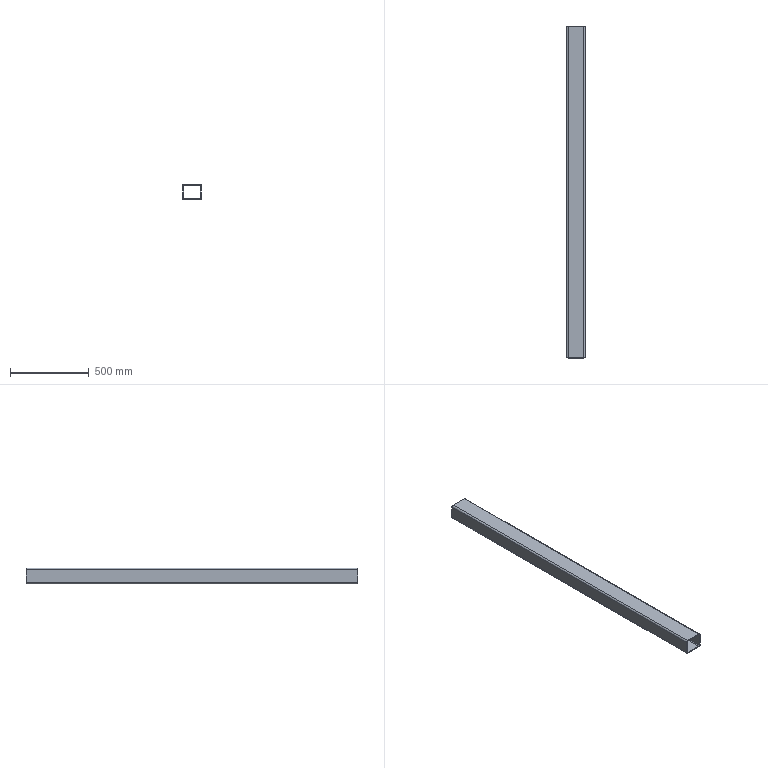Part | SolidWorks | features ExtruThin 1 | 1 solid | 18 faces | box 120 x 2114 x 100 mm | volume 5124111 mm3 | plane 10 | cylinder 8 | commonest cylinder face diameters 8 x4 20 x4
STEP:
#1=CARTESIAN_POINT('',(60.,1057.,-40.));
#2=VERTEX_POINT('',#1);
#3=CARTESIAN_POINT('',(50.,1057.,-50.));
#4=VERTEX_POINT('',#3);
#5=CARTESIAN_POINT('',(50.,1057.,-40.));
#6=DIRECTION('',(0.,1.,0.));
#7=DIRECTION('',(0.,0.,-1.));
#8=AXIS2_PLACEMENT_3D('',#5,#6,#7);
#9=CIRCLE('',#8,10.);
#10=EDGE_CURVE('',#2,#4,#9,.T.);
#11=ORIENTED_EDGE('',*,*,#10,.T.);
#12=CARTESIAN_POINT('',(-50.,1057.,-50.));
#13=VERTEX_POINT('',#12);
#14=CARTESIAN_POINT('',(-50.,1057.,-50.));
#15=DIRECTION('',(-1.,0.,0.));
#16=VECTOR('',#15,1000.);
#17=LINE('',#14,#16);
#18=EDGE_CURVE('',#4,#13,#17,.T.);
#19=ORIENTED_EDGE('',*,*,#18,.T.);
#20=CARTESIAN_POINT('',(-60.,1057.,-40.));
#21=VERTEX_POINT('',#20);
#22=CARTESIAN_POINT('',(-50.,1057.,-40.));
#23=DIRECTION('',(0.,1.,0.));
#24=DIRECTION('',(0.,0.,1.));
#25=AXIS2_PLACEMENT_3D('',#22,#23,#24);
#26=CIRCLE('',#25,10.);
#27=EDGE_CURVE('',#13,#21,#26,.T.);
#28=ORIENTED_EDGE('',*,*,#27,.T.);
#29=CARTESIAN_POINT('',(-60.,1057.,40.));
#30=VERTEX_POINT('',#29);
#31=CARTESIAN_POINT('',(-60.,1057.,-40.));
#32=DIRECTION('',(0.,0.,1.));
#33=VECTOR('',#32,1000.);
#34=LINE('',#31,#33);
#35=EDGE_CURVE('',#21,#30,#34,.T.);
#36=ORIENTED_EDGE('',*,*,#35,.T.);
#37=CARTESIAN_POINT('',(-50.,1057.,50.));
#38=VERTEX_POINT('',#37);
#39=CARTESIAN_POINT('',(-50.,1057.,40.));
#40=DIRECTION('',(0.,1.,0.));
#41=DIRECTION('',(0.,0.,1.));
#42=AXIS2_PLACEMENT_3D('',#39,#40,#41);
#43=CIRCLE('',#42,10.);
#44=EDGE_CURVE('',#30,#38,#43,.T.);
#45=ORIENTED_EDGE('',*,*,#44,.T.);
#46=CARTESIAN_POINT('',(50.,1057.,50.));
#47=VERTEX_POINT('',#46);
#48=CARTESIAN_POINT('',(-50.,1057.,50.));
#49=DIRECTION('',(1.,0.,0.));
#50=VECTOR('',#49,1000.);
#51=LINE('',#48,#50);
#52=EDGE_CURVE('',#38,#47,#51,.T.);
#53=ORIENTED_EDGE('',*,*,#52,.T.);
#54=CARTESIAN_POINT('',(60.,1057.,40.));
#55=VERTEX_POINT('',#54);
#56=CARTESIAN_POINT('',(50.,1057.,40.));
#57=DIRECTION('',(0.,1.,0.));
#58=DIRECTION('',(0.,0.,1.));
#59=AXIS2_PLACEMENT_3D('',#56,#57,#58);
#60=CIRCLE('',#59,10.);
#61=EDGE_CURVE('',#47,#55,#60,.T.);
#62=ORIENTED_EDGE('',*,*,#61,.T.);
#63=CARTESIAN_POINT('',(60.,1057.,-40.));
#64=DIRECTION('',(0.,0.,-1.));
#65=VECTOR('',#64,1000.);
#66=LINE('',#63,#65);
#67=EDGE_CURVE('',#55,#2,#66,.T.);
#68=ORIENTED_EDGE('',*,*,#67,.T.);
#69=EDGE_LOOP('',(#11,#19,#28,#36,#45,#53,#62,#68));
#70=FACE_OUTER_BOUND('',#69,.T.);
#71=CARTESIAN_POINT('',(50.,1057.,-44.));
#72=VERTEX_POINT('',#71);
#73=CARTESIAN_POINT('',(-50.,1057.,-44.));
#74=VERTEX_POINT('',#73);
#75=CARTESIAN_POINT('',(50.,1057.,-44.));
#76=DIRECTION('',(-1.,0.,0.));
#77=VECTOR('',#76,1000.);
#78=LINE('',#75,#77);
#79=EDGE_CURVE('',#72,#74,#78,.T.);
#80=ORIENTED_EDGE('',*,*,#79,.F.);
#81=CARTESIAN_POINT('',(54.,1057.,-40.));
#82=VERTEX_POINT('',#81);
#83=CARTESIAN_POINT('',(50.,1057.,-40.));
#84=DIRECTION('',(0.,1.,0.));
#85=DIRECTION('',(-1.,0.,0.));
#86=AXIS2_PLACEMENT_3D('',#83,#84,#85);
#87=CIRCLE('',#86,4.);
#88=EDGE_CURVE('',#82,#72,#87,.T.);
#89=ORIENTED_EDGE('',*,*,#88,.F.);
#90=CARTESIAN_POINT('',(54.,1057.,40.));
#91=VERTEX_POINT('',#90);
#92=CARTESIAN_POINT('',(54.,1057.,-40.));
#93=DIRECTION('',(0.,0.,-1.));
#94=VECTOR('',#93,1000.);
#95=LINE('',#92,#94);
#96=EDGE_CURVE('',#91,#82,#95,.T.);
#97=ORIENTED_EDGE('',*,*,#96,.F.);
#98=CARTESIAN_POINT('',(50.,1057.,44.));
#99=VERTEX_POINT('',#98);
#100=CARTESIAN_POINT('',(50.,1057.,40.));
#101=DIRECTION('',(0.,1.,0.));
#102=DIRECTION('',(-1.,0.,0.));
#103=AXIS2_PLACEMENT_3D('',#100,#101,#102);
#104=CIRCLE('',#103,4.);
#105=EDGE_CURVE('',#99,#91,#104,.T.);
#106=ORIENTED_EDGE('',*,*,#105,.F.);
#107=CARTESIAN_POINT('',(-50.,1057.,44.));
#108=VERTEX_POINT('',#107);
#109=CARTESIAN_POINT('',(50.,1057.,44.));
#110=DIRECTION('',(1.,0.,0.));
#111=VECTOR('',#110,1000.);
#112=LINE('',#109,#111);
#113=EDGE_CURVE('',#108,#99,#112,.T.);
#114=ORIENTED_EDGE('',*,*,#113,.F.);
#115=CARTESIAN_POINT('',(-54.,1057.,40.));
#116=VERTEX_POINT('',#115);
#117=CARTESIAN_POINT('',(-50.,1057.,40.));
#118=DIRECTION('',(0.,1.,0.));
#119=DIRECTION('',(-1.,0.,0.));
#120=AXIS2_PLACEMENT_3D('',#117,#118,#119);
#121=CIRCLE('',#120,4.);
#122=EDGE_CURVE('',#116,#108,#121,.T.);
#123=ORIENTED_EDGE('',*,*,#122,.F.);
#124=CARTESIAN_POINT('',(-54.,1057.,-40.));
#125=VERTEX_POINT('',#124);
#126=CARTESIAN_POINT('',(-54.,1057.,-40.));
#127=DIRECTION('',(0.,0.,1.));
#128=VECTOR('',#127,1000.);
#129=LINE('',#126,#128);
#130=EDGE_CURVE('',#125,#116,#129,.T.);
#131=ORIENTED_EDGE('',*,*,#130,.F.);
#132=CARTESIAN_POINT('',(-50.,1057.,-40.));
#133=DIRECTION('',(0.,1.,0.));
#134=DIRECTION('',(-1.,0.,0.));
#135=AXIS2_PLACEMENT_3D('',#132,#133,#134);
#136=CIRCLE('',#135,4.);
#137=EDGE_CURVE('',#74,#125,#136,.T.);
#138=ORIENTED_EDGE('',*,*,#137,.F.);
#139=EDGE_LOOP('',(#80,#89,#97,#106,#114,#123,#131,#138));
#140=FACE_BOUND('',#139,.T.);
#141=CARTESIAN_POINT('',(50.,1057.,-40.));
#142=DIRECTION('',(0.,1.,0.));
#143=DIRECTION('',(0.,0.,1.));
#144=AXIS2_PLACEMENT_3D('',#141,#142,#143);
#145=PLANE('',#144);
#146=ADVANCED_FACE('',(#70,#140),#145,.T.);
#147=CARTESIAN_POINT('',(60.,-1057.,-40.));
#148=VERTEX_POINT('',#147);
#149=CARTESIAN_POINT('',(50.,-1057.,-50.));
#150=VERTEX_POINT('',#149);
#151=CARTESIAN_POINT('',(50.,-1057.,-40.));
#152=DIRECTION('',(0.,1.,0.));
#153=DIRECTION('',(0.,0.,-1.));
#154=AXIS2_PLACEMENT_3D('',#151,#152,#153);
#155=CIRCLE('',#154,10.);
#156=EDGE_CURVE('',#148,#150,#155,.T.);
#157=ORIENTED_EDGE('',*,*,#156,.F.);
#158=CARTESIAN_POINT('',(60.,-1057.,40.));
#159=VERTEX_POINT('',#158);
#160=CARTESIAN_POINT('',(60.,-1057.,-40.));
#161=DIRECTION('',(0.,0.,-1.));
#162=VECTOR('',#161,1000.);
#163=LINE('',#160,#162);
#164=EDGE_CURVE('',#159,#148,#163,.T.);
#165=ORIENTED_EDGE('',*,*,#164,.F.);
#166=CARTESIAN_POINT('',(50.,-1057.,50.));
#167=VERTEX_POINT('',#166);
#168=CARTESIAN_POINT('',(50.,-1057.,40.));
#169=DIRECTION('',(0.,1.,0.));
#170=DIRECTION('',(0.,0.,1.));
#171=AXIS2_PLACEMENT_3D('',#168,#169,#170);
#172=CIRCLE('',#171,10.);
#173=EDGE_CURVE('',#167,#159,#172,.T.);
#174=ORIENTED_EDGE('',*,*,#173,.F.);
#175=CARTESIAN_POINT('',(-50.,-1057.,50.));
#176=VERTEX_POINT('',#175);
#177=CARTESIAN_POINT('',(-50.,-1057.,50.));
#178=DIRECTION('',(1.,0.,0.));
#179=VECTOR('',#178,1000.);
#180=LINE('',#177,#179);
#181=EDGE_CURVE('',#176,#167,#180,.T.);
#182=ORIENTED_EDGE('',*,*,#181,.F.);
#183=CARTESIAN_POINT('',(-60.,-1057.,40.));
#184=VERTEX_POINT('',#183);
#185=CARTESIAN_POINT('',(-50.,-1057.,40.));
#186=DIRECTION('',(0.,1.,0.));
#187=DIRECTION('',(0.,0.,1.));
#188=AXIS2_PLACEMENT_3D('',#185,#186,#187);
#189=CIRCLE('',#188,10.);
#190=EDGE_CURVE('',#184,#176,#189,.T.);
#191=ORIENTED_EDGE('',*,*,#190,.F.);
#192=CARTESIAN_POINT('',(-60.,-1057.,-40.));
#193=VERTEX_POINT('',#192);
#194=CARTESIAN_POINT('',(-60.,-1057.,-40.));
#195=DIRECTION('',(0.,0.,1.));
#196=VECTOR('',#195,1000.);
#197=LINE('',#194,#196);
#198=EDGE_CURVE('',#193,#184,#197,.T.);
#199=ORIENTED_EDGE('',*,*,#198,.F.);
#200=CARTESIAN_POINT('',(-50.,-1057.,-50.));
#201=VERTEX_POINT('',#200);
#202=CARTESIAN_POINT('',(-50.,-1057.,-40.));
#203=DIRECTION('',(0.,1.,0.));
#204=DIRECTION('',(0.,0.,1.));
#205=AXIS2_PLACEMENT_3D('',#202,#203,#204);
#206=CIRCLE('',#205,10.);
#207=EDGE_CURVE('',#201,#193,#206,.T.);
#208=ORIENTED_EDGE('',*,*,#207,.F.);
#209=CARTESIAN_POINT('',(-50.,-1057.,-50.));
#210=DIRECTION('',(-1.,0.,0.));
#211=VECTOR('',#210,1000.);
#212=LINE('',#209,#211);
#213=EDGE_CURVE('',#150,#201,#212,.T.);
#214=ORIENTED_EDGE('',*,*,#213,.F.);
#215=EDGE_LOOP('',(#157,#165,#174,#182,#191,#199,#208,#214));
#216=FACE_OUTER_BOUND('',#215,.T.);
#217=CARTESIAN_POINT('',(54.,-1057.,-40.));
#218=VERTEX_POINT('',#217);
#219=CARTESIAN_POINT('',(50.,-1057.,-44.));
#220=VERTEX_POINT('',#219);
#221=CARTESIAN_POINT('',(50.,-1057.,-40.));
#222=DIRECTION('',(0.,1.,0.));
#223=DIRECTION('',(-1.,0.,0.));
#224=AXIS2_PLACEMENT_3D('',#221,#222,#223);
#225=CIRCLE('',#224,4.);
#226=EDGE_CURVE('',#218,#220,#225,.T.);
#227=ORIENTED_EDGE('',*,*,#226,.T.);
#228=CARTESIAN_POINT('',(-50.,-1057.,-44.));
#229=VERTEX_POINT('',#228);
#230=CARTESIAN_POINT('',(50.,-1057.,-44.));
#231=DIRECTION('',(-1.,0.,0.));
#232=VECTOR('',#231,1000.);
#233=LINE('',#230,#232);
#234=EDGE_CURVE('',#220,#229,#233,.T.);
#235=ORIENTED_EDGE('',*,*,#234,.T.);
#236=CARTESIAN_POINT('',(-54.,-1057.,-40.));
#237=VERTEX_POINT('',#236);
#238=CARTESIAN_POINT('',(-50.,-1057.,-40.));
#239=DIRECTION('',(0.,1.,0.));
#240=DIRECTION('',(-1.,0.,0.));
#241=AXIS2_PLACEMENT_3D('',#238,#239,#240);
#242=CIRCLE('',#241,4.);
#243=EDGE_CURVE('',#229,#237,#242,.T.);
#244=ORIENTED_EDGE('',*,*,#243,.T.);
#245=CARTESIAN_POINT('',(-54.,-1057.,40.));
#246=VERTEX_POINT('',#245);
#247=CARTESIAN_POINT('',(-54.,-1057.,-40.));
#248=DIRECTION('',(0.,0.,1.));
#249=VECTOR('',#248,1000.);
#250=LINE('',#247,#249);
#251=EDGE_CURVE('',#237,#246,#250,.T.);
#252=ORIENTED_EDGE('',*,*,#251,.T.);
#253=CARTESIAN_POINT('',(-50.,-1057.,44.));
#254=VERTEX_POINT('',#253);
#255=CARTESIAN_POINT('',(-50.,-1057.,40.));
#256=DIRECTION('',(0.,1.,0.));
#257=DIRECTION('',(-1.,0.,0.));
#258=AXIS2_PLACEMENT_3D('',#255,#256,#257);
#259=CIRCLE('',#258,4.);
#260=EDGE_CURVE('',#246,#254,#259,.T.);
#261=ORIENTED_EDGE('',*,*,#260,.T.);
#262=CARTESIAN_POINT('',(50.,-1057.,44.));
#263=VERTEX_POINT('',#262);
#264=CARTESIAN_POINT('',(50.,-1057.,44.));
#265=DIRECTION('',(1.,0.,0.));
#266=VECTOR('',#265,1000.);
#267=LINE('',#264,#266);
#268=EDGE_CURVE('',#254,#263,#267,.T.);
#269=ORIENTED_EDGE('',*,*,#268,.T.);
#270=CARTESIAN_POINT('',(54.,-1057.,40.));
#271=VERTEX_POINT('',#270);
#272=CARTESIAN_POINT('',(50.,-1057.,40.));
#273=DIRECTION('',(0.,1.,0.));
#274=DIRECTION('',(-1.,0.,0.));
#275=AXIS2_PLACEMENT_3D('',#272,#273,#274);
#276=CIRCLE('',#275,4.);
#277=EDGE_CURVE('',#263,#271,#276,.T.);
#278=ORIENTED_EDGE('',*,*,#277,.T.);
#279=CARTESIAN_POINT('',(54.,-1057.,-40.));
#280=DIRECTION('',(0.,0.,-1.));
#281=VECTOR('',#280,1000.);
#282=LINE('',#279,#281);
#283=EDGE_CURVE('',#271,#218,#282,.T.);
#284=ORIENTED_EDGE('',*,*,#283,.T.);
#285=EDGE_LOOP('',(#227,#235,#244,#252,#261,#269,#278,#284));
#286=FACE_BOUND('',#285,.T.);
#287=CARTESIAN_POINT('',(50.,-1057.,-40.));
#288=DIRECTION('',(0.,1.,0.));
#289=DIRECTION('',(0.,0.,1.));
#290=AXIS2_PLACEMENT_3D('',#287,#288,#289);
#291=PLANE('',#290);
#292=ADVANCED_FACE('',(#216,#286),#291,.F.);
#293=ORIENTED_EDGE('',*,*,#156,.T.);
#294=CARTESIAN_POINT('',(50.,1057.,-50.));
#295=DIRECTION('',(0.,-1.,0.));
#296=VECTOR('',#295,1000.);
#297=LINE('',#294,#296);
#298=EDGE_CURVE('',#4,#150,#297,.T.);
#299=ORIENTED_EDGE('',*,*,#298,.F.);
#300=ORIENTED_EDGE('',*,*,#10,.F.);
#301=CARTESIAN_POINT('',(60.,1057.,-40.));
#302=DIRECTION('',(0.,-1.,0.));
#303=VECTOR('',#302,1000.);
#304=LINE('',#301,#303);
#305=EDGE_CURVE('',#2,#148,#304,.T.);
#306=ORIENTED_EDGE('',*,*,#305,.T.);
#307=EDGE_LOOP('',(#293,#299,#300,#306));
#308=FACE_OUTER_BOUND('',#307,.T.);
#309=CARTESIAN_POINT('',(50.,1057.,-40.));
#310=DIRECTION('',(0.,-1.,0.));
#311=DIRECTION('',(0.,0.,-1.));
#312=AXIS2_PLACEMENT_3D('',#309,#310,#311);
#313=CYLINDRICAL_SURFACE('',#312,10.);
#314=ADVANCED_FACE('',(#308),#313,.T.);
#315=ORIENTED_EDGE('',*,*,#213,.T.);
#316=CARTESIAN_POINT('',(-50.,1057.,-50.));
#317=DIRECTION('',(0.,-1.,0.));
#318=VECTOR('',#317,1000.);
#319=LINE('',#316,#318);
#320=EDGE_CURVE('',#13,#201,#319,.T.);
#321=ORIENTED_EDGE('',*,*,#320,.F.);
#322=ORIENTED_EDGE('',*,*,#18,.F.);
#323=ORIENTED_EDGE('',*,*,#298,.T.);
#324=EDGE_LOOP('',(#315,#321,#322,#323));
#325=FACE_OUTER_BOUND('',#324,.T.);
#326=CARTESIAN_POINT('',(-50.,1057.,-50.));
#327=DIRECTION('',(0.,0.,1.));
#328=DIRECTION('',(1.,0.,0.));
#329=AXIS2_PLACEMENT_3D('',#326,#327,#328);
#330=PLANE('',#329);
#331=ADVANCED_FACE('',(#325),#330,.F.);
#332=ORIENTED_EDGE('',*,*,#207,.T.);
#333=CARTESIAN_POINT('',(-60.,1057.,-40.));
#334=DIRECTION('',(0.,-1.,0.));
#335=VECTOR('',#334,1000.);
#336=LINE('',#333,#335);
#337=EDGE_CURVE('',#21,#193,#336,.T.);
#338=ORIENTED_EDGE('',*,*,#337,.F.);
#339=ORIENTED_EDGE('',*,*,#27,.F.);
#340=ORIENTED_EDGE('',*,*,#320,.T.);
#341=EDGE_LOOP('',(#332,#338,#339,#340));
#342=FACE_OUTER_BOUND('',#341,.T.);
#343=CARTESIAN_POINT('',(-50.,1057.,-40.));
#344=DIRECTION('',(0.,-1.,0.));
#345=DIRECTION('',(0.,0.,-1.));
#346=AXIS2_PLACEMENT_3D('',#343,#344,#345);
#347=CYLINDRICAL_SURFACE('',#346,10.);
#348=ADVANCED_FACE('',(#342),#347,.T.);
#349=ORIENTED_EDGE('',*,*,#198,.T.);
#350=CARTESIAN_POINT('',(-60.,1057.,40.));
#351=DIRECTION('',(0.,-1.,0.));
#352=VECTOR('',#351,1000.);
#353=LINE('',#350,#352);
#354=EDGE_CURVE('',#30,#184,#353,.T.);
#355=ORIENTED_EDGE('',*,*,#354,.F.);
#356=ORIENTED_EDGE('',*,*,#35,.F.);
#357=ORIENTED_EDGE('',*,*,#337,.T.);
#358=EDGE_LOOP('',(#349,#355,#356,#357));
#359=FACE_OUTER_BOUND('',#358,.T.);
#360=CARTESIAN_POINT('',(-60.,1057.,-40.));
#361=DIRECTION('',(1.,0.,0.));
#362=DIRECTION('',(0.,0.,-1.));
#363=AXIS2_PLACEMENT_3D('',#360,#361,#362);
#364=PLANE('',#363);
#365=ADVANCED_FACE('',(#359),#364,.F.);
#366=ORIENTED_EDGE('',*,*,#190,.T.);
#367=CARTESIAN_POINT('',(-50.,1057.,50.));
#368=DIRECTION('',(0.,-1.,0.));
#369=VECTOR('',#368,1000.);
#370=LINE('',#367,#369);
#371=EDGE_CURVE('',#38,#176,#370,.T.);
#372=ORIENTED_EDGE('',*,*,#371,.F.);
#373=ORIENTED_EDGE('',*,*,#44,.F.);
#374=ORIENTED_EDGE('',*,*,#354,.T.);
#375=EDGE_LOOP('',(#366,#372,#373,#374));
#376=FACE_OUTER_BOUND('',#375,.T.);
#377=CARTESIAN_POINT('',(-50.,1057.,40.));
#378=DIRECTION('',(0.,-1.,0.));
#379=DIRECTION('',(0.,0.,-1.));
#380=AXIS2_PLACEMENT_3D('',#377,#378,#379);
#381=CYLINDRICAL_SURFACE('',#380,10.);
#382=ADVANCED_FACE('',(#376),#381,.T.);
#383=ORIENTED_EDGE('',*,*,#181,.T.);
#384=CARTESIAN_POINT('',(50.,1057.,50.));
#385=DIRECTION('',(0.,-1.,0.));
#386=VECTOR('',#385,1000.);
#387=LINE('',#384,#386);
#388=EDGE_CURVE('',#47,#167,#387,.T.);
#389=ORIENTED_EDGE('',*,*,#388,.F.);
#390=ORIENTED_EDGE('',*,*,#52,.F.);
#391=ORIENTED_EDGE('',*,*,#371,.T.);
#392=EDGE_LOOP('',(#383,#389,#390,#391));
#393=FACE_OUTER_BOUND('',#392,.T.);
#394=CARTESIAN_POINT('',(-50.,1057.,50.));
#395=DIRECTION('',(0.,0.,-1.));
#396=DIRECTION('',(-1.,0.,0.));
#397=AXIS2_PLACEMENT_3D('',#394,#395,#396);
#398=PLANE('',#397);
#399=ADVANCED_FACE('',(#393),#398,.F.);
#400=ORIENTED_EDGE('',*,*,#173,.T.);
#401=CARTESIAN_POINT('',(60.,1057.,40.));
#402=DIRECTION('',(0.,-1.,0.));
#403=VECTOR('',#402,1000.);
#404=LINE('',#401,#403);
#405=EDGE_CURVE('',#55,#159,#404,.T.);
#406=ORIENTED_EDGE('',*,*,#405,.F.);
#407=ORIENTED_EDGE('',*,*,#61,.F.);
#408=ORIENTED_EDGE('',*,*,#388,.T.);
#409=EDGE_LOOP('',(#400,#406,#407,#408));
#410=FACE_OUTER_BOUND('',#409,.T.);
#411=CARTESIAN_POINT('',(50.,1057.,40.));
#412=DIRECTION('',(0.,-1.,0.));
#413=DIRECTION('',(0.,0.,-1.));
#414=AXIS2_PLACEMENT_3D('',#411,#412,#413);
#415=CYLINDRICAL_SURFACE('',#414,10.);
#416=ADVANCED_FACE('',(#410),#415,.T.);
#417=ORIENTED_EDGE('',*,*,#164,.T.);
#418=ORIENTED_EDGE('',*,*,#305,.F.);
#419=ORIENTED_EDGE('',*,*,#67,.F.);
#420=ORIENTED_EDGE('',*,*,#405,.T.);
#421=EDGE_LOOP('',(#417,#418,#419,#420));
#422=FACE_OUTER_BOUND('',#421,.T.);
#423=CARTESIAN_POINT('',(60.,1057.,-40.));
#424=DIRECTION('',(-1.,0.,0.));
#425=DIRECTION('',(0.,0.,1.));
#426=AXIS2_PLACEMENT_3D('',#423,#424,#425);
#427=PLANE('',#426);
#428=ADVANCED_FACE('',(#422),#427,.F.);
#429=ORIENTED_EDGE('',*,*,#226,.F.);
#430=CARTESIAN_POINT('',(54.,1057.,-40.));
#431=DIRECTION('',(0.,-1.,0.));
#432=VECTOR('',#431,1000.);
#433=LINE('',#430,#432);
#434=EDGE_CURVE('',#82,#218,#433,.T.);
#435=ORIENTED_EDGE('',*,*,#434,.F.);
#436=ORIENTED_EDGE('',*,*,#88,.T.);
#437=CARTESIAN_POINT('',(50.,1057.,-44.));
#438=DIRECTION('',(0.,-1.,0.));
#439=VECTOR('',#438,1000.);
#440=LINE('',#437,#439);
#441=EDGE_CURVE('',#72,#220,#440,.T.);
#442=ORIENTED_EDGE('',*,*,#441,.T.);
#443=EDGE_LOOP('',(#429,#435,#436,#442));
#444=FACE_OUTER_BOUND('',#443,.T.);
#445=CARTESIAN_POINT('',(50.,1057.,-40.));
#446=DIRECTION('',(0.,-1.,0.));
#447=DIRECTION('',(0.,0.,-1.));
#448=AXIS2_PLACEMENT_3D('',#445,#446,#447);
#449=CYLINDRICAL_SURFACE('',#448,4.);
#450=ADVANCED_FACE('',(#444),#449,.F.);
#451=ORIENTED_EDGE('',*,*,#234,.F.);
#452=ORIENTED_EDGE('',*,*,#441,.F.);
#453=ORIENTED_EDGE('',*,*,#79,.T.);
#454=CARTESIAN_POINT('',(-50.,1057.,-44.));
#455=DIRECTION('',(0.,-1.,0.));
#456=VECTOR('',#455,1000.);
#457=LINE('',#454,#456);
#458=EDGE_CURVE('',#74,#229,#457,.T.);
#459=ORIENTED_EDGE('',*,*,#458,.T.);
#460=EDGE_LOOP('',(#451,#452,#453,#459));
#461=FACE_OUTER_BOUND('',#460,.T.);
#462=CARTESIAN_POINT('',(50.,1057.,-44.));
#463=DIRECTION('',(0.,0.,1.));
#464=DIRECTION('',(1.,0.,0.));
#465=AXIS2_PLACEMENT_3D('',#462,#463,#464);
#466=PLANE('',#465);
#467=ADVANCED_FACE('',(#461),#466,.T.);
#468=ORIENTED_EDGE('',*,*,#243,.F.);
#469=ORIENTED_EDGE('',*,*,#458,.F.);
#470=ORIENTED_EDGE('',*,*,#137,.T.);
#471=CARTESIAN_POINT('',(-54.,1057.,-40.));
#472=DIRECTION('',(0.,-1.,0.));
#473=VECTOR('',#472,1000.);
#474=LINE('',#471,#473);
#475=EDGE_CURVE('',#125,#237,#474,.T.);
#476=ORIENTED_EDGE('',*,*,#475,.T.);
#477=EDGE_LOOP('',(#468,#469,#470,#476));
#478=FACE_OUTER_BOUND('',#477,.T.);
#479=CARTESIAN_POINT('',(-50.,1057.,-40.));
#480=DIRECTION('',(0.,-1.,0.));
#481=DIRECTION('',(0.,0.,-1.));
#482=AXIS2_PLACEMENT_3D('',#479,#480,#481);
#483=CYLINDRICAL_SURFACE('',#482,4.);
#484=ADVANCED_FACE('',(#478),#483,.F.);
#485=ORIENTED_EDGE('',*,*,#251,.F.);
#486=ORIENTED_EDGE('',*,*,#475,.F.);
#487=ORIENTED_EDGE('',*,*,#130,.T.);
#488=CARTESIAN_POINT('',(-54.,1057.,40.));
#489=DIRECTION('',(0.,-1.,0.));
#490=VECTOR('',#489,1000.);
#491=LINE('',#488,#490);
#492=EDGE_CURVE('',#116,#246,#491,.T.);
#493=ORIENTED_EDGE('',*,*,#492,.T.);
#494=EDGE_LOOP('',(#485,#486,#487,#493));
#495=FACE_OUTER_BOUND('',#494,.T.);
#496=CARTESIAN_POINT('',(-54.,1057.,-40.));
#497=DIRECTION('',(1.,0.,0.));
#498=DIRECTION('',(0.,0.,-1.));
#499=AXIS2_PLACEMENT_3D('',#496,#497,#498);
#500=PLANE('',#499);
#501=ADVANCED_FACE('',(#495),#500,.T.);
#502=ORIENTED_EDGE('',*,*,#260,.F.);
#503=ORIENTED_EDGE('',*,*,#492,.F.);
#504=ORIENTED_EDGE('',*,*,#122,.T.);
#505=CARTESIAN_POINT('',(-50.,1057.,44.));
#506=DIRECTION('',(0.,-1.,0.));
#507=VECTOR('',#506,1000.);
#508=LINE('',#505,#507);
#509=EDGE_CURVE('',#108,#254,#508,.T.);
#510=ORIENTED_EDGE('',*,*,#509,.T.);
#511=EDGE_LOOP('',(#502,#503,#504,#510));
#512=FACE_OUTER_BOUND('',#511,.T.);
#513=CARTESIAN_POINT('',(-50.,1057.,40.));
#514=DIRECTION('',(0.,-1.,0.));
#515=DIRECTION('',(0.,0.,-1.));
#516=AXIS2_PLACEMENT_3D('',#513,#514,#515);
#517=CYLINDRICAL_SURFACE('',#516,4.);
#518=ADVANCED_FACE('',(#512),#517,.F.);
#519=ORIENTED_EDGE('',*,*,#268,.F.);
#520=ORIENTED_EDGE('',*,*,#509,.F.);
#521=ORIENTED_EDGE('',*,*,#113,.T.);
#522=CARTESIAN_POINT('',(50.,1057.,44.));
#523=DIRECTION('',(0.,-1.,0.));
#524=VECTOR('',#523,1000.);
#525=LINE('',#522,#524);
#526=EDGE_CURVE('',#99,#263,#525,.T.);
#527=ORIENTED_EDGE('',*,*,#526,.T.);
#528=EDGE_LOOP('',(#519,#520,#521,#527));
#529=FACE_OUTER_BOUND('',#528,.T.);
#530=CARTESIAN_POINT('',(50.,1057.,44.));
#531=DIRECTION('',(0.,0.,-1.));
#532=DIRECTION('',(-1.,0.,0.));
#533=AXIS2_PLACEMENT_3D('',#530,#531,#532);
#534=PLANE('',#533);
#535=ADVANCED_FACE('',(#529),#534,.T.);
#536=ORIENTED_EDGE('',*,*,#277,.F.);
#537=ORIENTED_EDGE('',*,*,#526,.F.);
#538=ORIENTED_EDGE('',*,*,#105,.T.);
#539=CARTESIAN_POINT('',(54.,1057.,40.));
#540=DIRECTION('',(0.,-1.,0.));
#541=VECTOR('',#540,1000.);
#542=LINE('',#539,#541);
#543=EDGE_CURVE('',#91,#271,#542,.T.);
#544=ORIENTED_EDGE('',*,*,#543,.T.);
#545=EDGE_LOOP('',(#536,#537,#538,#544));
#546=FACE_OUTER_BOUND('',#545,.T.);
#547=CARTESIAN_POINT('',(50.,1057.,40.));
#548=DIRECTION('',(0.,-1.,0.));
#549=DIRECTION('',(0.,0.,-1.));
#550=AXIS2_PLACEMENT_3D('',#547,#548,#549);
#551=CYLINDRICAL_SURFACE('',#550,4.);
#552=ADVANCED_FACE('',(#546),#551,.F.);
#553=ORIENTED_EDGE('',*,*,#283,.F.);
#554=ORIENTED_EDGE('',*,*,#543,.F.);
#555=ORIENTED_EDGE('',*,*,#96,.T.);
#556=ORIENTED_EDGE('',*,*,#434,.T.);
#557=EDGE_LOOP('',(#553,#554,#555,#556));
#558=FACE_OUTER_BOUND('',#557,.T.);
#559=CARTESIAN_POINT('',(54.,1057.,-40.));
#560=DIRECTION('',(-1.,0.,0.));
#561=DIRECTION('',(0.,0.,1.));
#562=AXIS2_PLACEMENT_3D('',#559,#560,#561);
#563=PLANE('',#562);
#564=ADVANCED_FACE('',(#558),#563,.T.);
#565=CLOSED_SHELL('',(#146,#292,#314,#331,#348,#365,#382,#399,#416,#428,#450,#467,#484,#501,#518,#535,#552,#564));
#566=MANIFOLD_SOLID_BREP('',#565);
#567=CARTESIAN_POINT('',(0.,0.,0.));
#568=DIRECTION('',(0.,0.,1.));
#569=DIRECTION('',(1.,0.,0.));
#570=AXIS2_PLACEMENT_3D('',#567,#568,#569);
#571=(LENGTH_UNIT()NAMED_UNIT(*)SI_UNIT(.MILLI.,.METRE.));
#572=UNCERTAINTY_MEASURE_WITH_UNIT(LENGTH_MEASURE(0.00001),#571,'','');
#573=(NAMED_UNIT(*)PLANE_ANGLE_UNIT()SI_UNIT($,.RADIAN.));
#574=(NAMED_UNIT(*)SI_UNIT($,.STERADIAN.)SOLID_ANGLE_UNIT());
#575=(GEOMETRIC_REPRESENTATION_CONTEXT(3)GLOBAL_UNCERTAINTY_ASSIGNED_CONTEXT((#572))GLOBAL_UNIT_ASSIGNED_CONTEXT((#571,#573,#574))REPRESENTATION_CONTEXT('',''));
#576=ADVANCED_BREP_SHAPE_REPRESENTATION('',(#566,#570),#575);